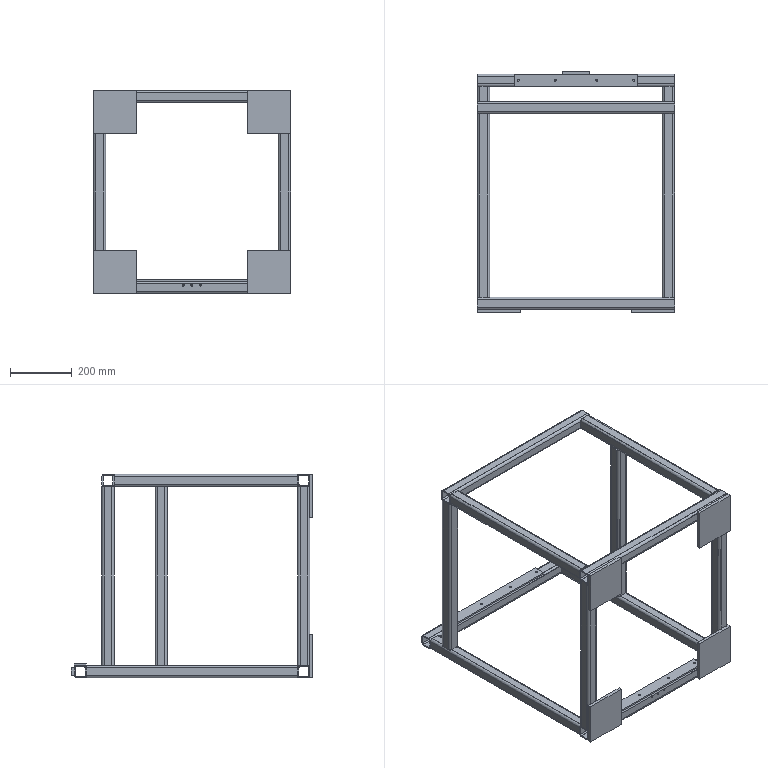Part | STEP file | 19 solids | 304 faces | box 640 x 785 x 660 mm | volume 4940885 mm3 | plane 162 | cylinder 142 | commonest cylinder face diameters 8 x48 16 x48 6.8 x38 5 x8